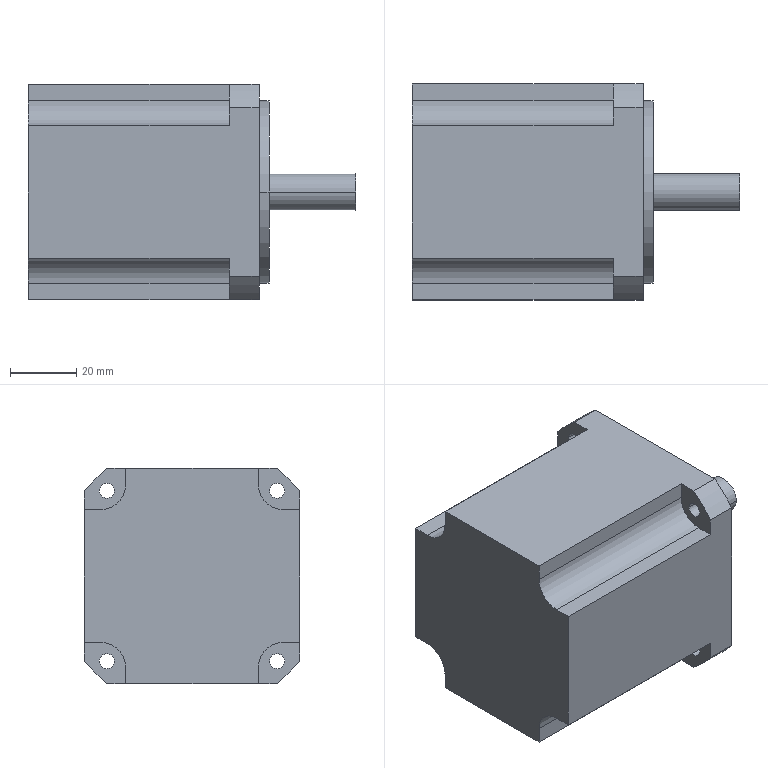Part | STEP file | 2026.6.15-Main Assembly图.sldasm-Part-113 | 1 solid | 40 faces | box 98.5 x 65 x 65 mm | volume 266939 mm3 | cylinder 20 | plane 20 | commonest cylinder face diameters 4.5 x8 15 x4 82.5 x4 11 x2 55 x2
STEP:
#1=CARTESIAN_POINT('',(-1698.224,586.801,4296.167));
#2=VERTEX_POINT('',#1);
#3=CARTESIAN_POINT('',(-1698.224,531.801,4296.167));
#4=VERTEX_POINT('',#3);
#5=CARTESIAN_POINT('',(-1698.224,559.301,4296.167));
#6=DIRECTION('',(1.,0.,0.));
#7=DIRECTION('',(0.,-1.,0.));
#8=AXIS2_PLACEMENT_3D('',#5,#6,#7);
#9=CIRCLE('',#8,27.5);
#10=EDGE_CURVE('',#2,#4,#9,.T.);
#11=ORIENTED_EDGE('',*,*,#10,.T.);
#12=CARTESIAN_POINT('',(-1695.224,531.801,4296.167));
#13=VERTEX_POINT('',#12);
#14=CARTESIAN_POINT('',(-1698.224,531.801,4296.167));
#15=DIRECTION('',(1.,0.,0.));
#16=VECTOR('',#15,1000.);
#17=LINE('',#14,#16);
#18=EDGE_CURVE('',#4,#13,#17,.T.);
#19=ORIENTED_EDGE('',*,*,#18,.T.);
#20=CARTESIAN_POINT('',(-1695.224,586.801,4296.167));
#21=VERTEX_POINT('',#20);
#22=CARTESIAN_POINT('',(-1695.224,559.301,4296.167));
#23=DIRECTION('',(1.,0.,0.));
#24=DIRECTION('',(0.,-1.,0.));
#25=AXIS2_PLACEMENT_3D('',#22,#23,#24);
#26=CIRCLE('',#25,27.5);
#27=EDGE_CURVE('',#21,#13,#26,.T.);
#28=ORIENTED_EDGE('',*,*,#27,.F.);
#29=CARTESIAN_POINT('',(-1698.224,586.801,4296.167));
#30=DIRECTION('',(1.,0.,0.));
#31=VECTOR('',#30,1000.);
#32=LINE('',#29,#31);
#33=EDGE_CURVE('',#2,#21,#32,.T.);
#34=ORIENTED_EDGE('',*,*,#33,.F.);
#35=EDGE_LOOP('',(#11,#19,#28,#34));
#36=FACE_OUTER_BOUND('',#35,.T.);
#37=CARTESIAN_POINT('',(-1698.224,559.301,4296.167));
#38=DIRECTION('',(1.,0.,0.));
#39=DIRECTION('',(0.,1.,0.));
#40=AXIS2_PLACEMENT_3D('',#37,#38,#39);
#41=CYLINDRICAL_SURFACE('',#40,27.5);
#42=ADVANCED_FACE('',(#36),#41,.T.);
#43=CARTESIAN_POINT('',(-1707.224,531.419,4270.534));
#44=VERTEX_POINT('',#43);
#45=CARTESIAN_POINT('',(-1707.224,535.919,4270.534));
#46=VERTEX_POINT('',#45);
#47=CARTESIAN_POINT('',(-1707.224,533.669,4270.534));
#48=DIRECTION('',(1.,0.,0.));
#49=DIRECTION('',(0.,1.,0.));
#50=AXIS2_PLACEMENT_3D('',#47,#48,#49);
#51=CIRCLE('',#50,2.25);
#52=EDGE_CURVE('',#44,#46,#51,.T.);
#53=ORIENTED_EDGE('',*,*,#52,.F.);
#54=CARTESIAN_POINT('',(-1698.224,531.419,4270.534));
#55=VERTEX_POINT('',#54);
#56=CARTESIAN_POINT('',(-1707.224,531.419,4270.534));
#57=DIRECTION('',(1.,0.,0.));
#58=VECTOR('',#57,1000.);
#59=LINE('',#56,#58);
#60=EDGE_CURVE('',#44,#55,#59,.T.);
#61=ORIENTED_EDGE('',*,*,#60,.T.);
#62=CARTESIAN_POINT('',(-1698.224,535.919,4270.534));
#63=VERTEX_POINT('',#62);
#64=CARTESIAN_POINT('',(-1698.224,533.669,4270.534));
#65=DIRECTION('',(1.,0.,0.));
#66=DIRECTION('',(0.,1.,0.));
#67=AXIS2_PLACEMENT_3D('',#64,#65,#66);
#68=CIRCLE('',#67,2.25);
#69=EDGE_CURVE('',#55,#63,#68,.T.);
#70=ORIENTED_EDGE('',*,*,#69,.T.);
#71=CARTESIAN_POINT('',(-1707.224,535.919,4270.534));
#72=DIRECTION('',(1.,0.,0.));
#73=VECTOR('',#72,1000.);
#74=LINE('',#71,#73);
#75=EDGE_CURVE('',#46,#63,#74,.T.);
#76=ORIENTED_EDGE('',*,*,#75,.F.);
#77=EDGE_LOOP('',(#53,#61,#70,#76));
#78=FACE_OUTER_BOUND('',#77,.T.);
#79=CARTESIAN_POINT('',(-1707.224,533.669,4270.534));
#80=DIRECTION('',(1.,0.,0.));
#81=DIRECTION('',(0.,1.,0.));
#82=AXIS2_PLACEMENT_3D('',#79,#80,#81);
#83=CYLINDRICAL_SURFACE('',#82,2.25);
#84=ADVANCED_FACE('',(#78),#83,.F.);
#85=CARTESIAN_POINT('',(-1707.224,582.684,4321.799));
#86=VERTEX_POINT('',#85);
#87=CARTESIAN_POINT('',(-1707.224,587.184,4321.799));
#88=VERTEX_POINT('',#87);
#89=CARTESIAN_POINT('',(-1707.224,584.934,4321.799));
#90=DIRECTION('',(1.,0.,0.));
#91=DIRECTION('',(0.,1.,0.));
#92=AXIS2_PLACEMENT_3D('',#89,#90,#91);
#93=CIRCLE('',#92,2.25);
#94=EDGE_CURVE('',#86,#88,#93,.T.);
#95=ORIENTED_EDGE('',*,*,#94,.F.);
#96=CARTESIAN_POINT('',(-1698.224,582.684,4321.799));
#97=VERTEX_POINT('',#96);
#98=CARTESIAN_POINT('',(-1707.224,582.684,4321.799));
#99=DIRECTION('',(1.,0.,0.));
#100=VECTOR('',#99,1000.);
#101=LINE('',#98,#100);
#102=EDGE_CURVE('',#86,#97,#101,.T.);
#103=ORIENTED_EDGE('',*,*,#102,.T.);
#104=CARTESIAN_POINT('',(-1698.224,587.184,4321.799));
#105=VERTEX_POINT('',#104);
#106=CARTESIAN_POINT('',(-1698.224,584.934,4321.799));
#107=DIRECTION('',(1.,0.,0.));
#108=DIRECTION('',(0.,1.,0.));
#109=AXIS2_PLACEMENT_3D('',#106,#107,#108);
#110=CIRCLE('',#109,2.25);
#111=EDGE_CURVE('',#97,#105,#110,.T.);
#112=ORIENTED_EDGE('',*,*,#111,.T.);
#113=CARTESIAN_POINT('',(-1707.224,587.184,4321.799));
#114=DIRECTION('',(1.,0.,0.));
#115=VECTOR('',#114,1000.);
#116=LINE('',#113,#115);
#117=EDGE_CURVE('',#88,#105,#116,.T.);
#118=ORIENTED_EDGE('',*,*,#117,.F.);
#119=EDGE_LOOP('',(#95,#103,#112,#118));
#120=FACE_OUTER_BOUND('',#119,.T.);
#121=CARTESIAN_POINT('',(-1707.224,584.934,4321.799));
#122=DIRECTION('',(1.,0.,0.));
#123=DIRECTION('',(0.,1.,0.));
#124=AXIS2_PLACEMENT_3D('',#121,#122,#123);
#125=CYLINDRICAL_SURFACE('',#124,2.25);
#126=ADVANCED_FACE('',(#120),#125,.F.);
#127=CARTESIAN_POINT('',(-1707.224,531.419,4321.799));
#128=VERTEX_POINT('',#127);
#129=CARTESIAN_POINT('',(-1707.224,535.919,4321.799));
#130=VERTEX_POINT('',#129);
#131=CARTESIAN_POINT('',(-1707.224,533.669,4321.799));
#132=DIRECTION('',(1.,0.,0.));
#133=DIRECTION('',(0.,1.,0.));
#134=AXIS2_PLACEMENT_3D('',#131,#132,#133);
#135=CIRCLE('',#134,2.25);
#136=EDGE_CURVE('',#128,#130,#135,.T.);
#137=ORIENTED_EDGE('',*,*,#136,.F.);
#138=CARTESIAN_POINT('',(-1698.224,531.419,4321.799));
#139=VERTEX_POINT('',#138);
#140=CARTESIAN_POINT('',(-1707.224,531.419,4321.799));
#141=DIRECTION('',(1.,0.,0.));
#142=VECTOR('',#141,1000.);
#143=LINE('',#140,#142);
#144=EDGE_CURVE('',#128,#139,#143,.T.);
#145=ORIENTED_EDGE('',*,*,#144,.T.);
#146=CARTESIAN_POINT('',(-1698.224,535.919,4321.799));
#147=VERTEX_POINT('',#146);
#148=CARTESIAN_POINT('',(-1698.224,533.669,4321.799));
#149=DIRECTION('',(1.,0.,0.));
#150=DIRECTION('',(0.,1.,0.));
#151=AXIS2_PLACEMENT_3D('',#148,#149,#150);
#152=CIRCLE('',#151,2.25);
#153=EDGE_CURVE('',#139,#147,#152,.T.);
#154=ORIENTED_EDGE('',*,*,#153,.T.);
#155=CARTESIAN_POINT('',(-1707.224,535.919,4321.799));
#156=DIRECTION('',(1.,0.,0.));
#157=VECTOR('',#156,1000.);
#158=LINE('',#155,#157);
#159=EDGE_CURVE('',#130,#147,#158,.T.);
#160=ORIENTED_EDGE('',*,*,#159,.F.);
#161=EDGE_LOOP('',(#137,#145,#154,#160));
#162=FACE_OUTER_BOUND('',#161,.T.);
#163=CARTESIAN_POINT('',(-1707.224,533.669,4321.799));
#164=DIRECTION('',(1.,0.,0.));
#165=DIRECTION('',(0.,1.,0.));
#166=AXIS2_PLACEMENT_3D('',#163,#164,#165);
#167=CYLINDRICAL_SURFACE('',#166,2.25);
#168=ADVANCED_FACE('',(#162),#167,.F.);
#169=CARTESIAN_POINT('',(-1707.224,582.684,4270.534));
#170=VERTEX_POINT('',#169);
#171=CARTESIAN_POINT('',(-1707.224,587.184,4270.534));
#172=VERTEX_POINT('',#171);
#173=CARTESIAN_POINT('',(-1707.224,584.934,4270.534));
#174=DIRECTION('',(1.,0.,0.));
#175=DIRECTION('',(0.,1.,0.));
#176=AXIS2_PLACEMENT_3D('',#173,#174,#175);
#177=CIRCLE('',#176,2.25);
#178=EDGE_CURVE('',#170,#172,#177,.T.);
#179=ORIENTED_EDGE('',*,*,#178,.F.);
#180=CARTESIAN_POINT('',(-1698.224,582.684,4270.534));
#181=VERTEX_POINT('',#180);
#182=CARTESIAN_POINT('',(-1707.224,582.684,4270.534));
#183=DIRECTION('',(1.,0.,0.));
#184=VECTOR('',#183,1000.);
#185=LINE('',#182,#184);
#186=EDGE_CURVE('',#170,#181,#185,.T.);
#187=ORIENTED_EDGE('',*,*,#186,.T.);
#188=CARTESIAN_POINT('',(-1698.224,587.184,4270.534));
#189=VERTEX_POINT('',#188);
#190=CARTESIAN_POINT('',(-1698.224,584.934,4270.534));
#191=DIRECTION('',(1.,0.,0.));
#192=DIRECTION('',(0.,1.,0.));
#193=AXIS2_PLACEMENT_3D('',#190,#191,#192);
#194=CIRCLE('',#193,2.25);
#195=EDGE_CURVE('',#181,#189,#194,.T.);
#196=ORIENTED_EDGE('',*,*,#195,.T.);
#197=CARTESIAN_POINT('',(-1707.224,587.184,4270.534));
#198=DIRECTION('',(1.,0.,0.));
#199=VECTOR('',#198,1000.);
#200=LINE('',#197,#199);
#201=EDGE_CURVE('',#172,#189,#200,.T.);
#202=ORIENTED_EDGE('',*,*,#201,.F.);
#203=EDGE_LOOP('',(#179,#187,#196,#202));
#204=FACE_OUTER_BOUND('',#203,.T.);
#205=CARTESIAN_POINT('',(-1707.224,584.934,4270.534));
#206=DIRECTION('',(1.,0.,0.));
#207=DIRECTION('',(0.,1.,0.));
#208=AXIS2_PLACEMENT_3D('',#205,#206,#207);
#209=CYLINDRICAL_SURFACE('',#208,2.25);
#210=ADVANCED_FACE('',(#204),#209,.F.);
#211=CARTESIAN_POINT('',(-1669.224,553.801,4296.167));
#212=VERTEX_POINT('',#211);
#213=CARTESIAN_POINT('',(-1669.224,564.801,4296.167));
#214=VERTEX_POINT('',#213);
#215=CARTESIAN_POINT('',(-1669.224,559.301,4296.167));
#216=DIRECTION('',(-1.,0.,0.));
#217=DIRECTION('',(0.,0.,1.));
#218=AXIS2_PLACEMENT_3D('',#215,#216,#217);
#219=CIRCLE('',#218,5.5);
#220=EDGE_CURVE('',#212,#214,#219,.T.);
#221=ORIENTED_EDGE('',*,*,#220,.T.);
#222=CARTESIAN_POINT('',(-1695.224,564.801,4296.167));
#223=VERTEX_POINT('',#222);
#224=CARTESIAN_POINT('',(-1669.224,564.801,4296.167));
#225=DIRECTION('',(-1.,0.,0.));
#226=VECTOR('',#225,1000.);
#227=LINE('',#224,#226);
#228=EDGE_CURVE('',#214,#223,#227,.T.);
#229=ORIENTED_EDGE('',*,*,#228,.T.);
#230=CARTESIAN_POINT('',(-1695.224,553.801,4296.167));
#231=VERTEX_POINT('',#230);
#232=CARTESIAN_POINT('',(-1695.224,559.301,4296.167));
#233=DIRECTION('',(-1.,0.,0.));
#234=DIRECTION('',(0.,0.,1.));
#235=AXIS2_PLACEMENT_3D('',#232,#233,#234);
#236=CIRCLE('',#235,5.5);
#237=EDGE_CURVE('',#231,#223,#236,.T.);
#238=ORIENTED_EDGE('',*,*,#237,.F.);
#239=CARTESIAN_POINT('',(-1669.224,553.801,4296.167));
#240=DIRECTION('',(-1.,0.,0.));
#241=VECTOR('',#240,1000.);
#242=LINE('',#239,#241);
#243=EDGE_CURVE('',#212,#231,#242,.T.);
#244=ORIENTED_EDGE('',*,*,#243,.F.);
#245=EDGE_LOOP('',(#221,#229,#238,#244));
#246=FACE_OUTER_BOUND('',#245,.T.);
#247=CARTESIAN_POINT('',(-1669.224,559.301,4296.167));
#248=DIRECTION('',(-1.,0.,0.));
#249=DIRECTION('',(0.,-1.,0.));
#250=AXIS2_PLACEMENT_3D('',#247,#248,#249);
#251=CYLINDRICAL_SURFACE('',#250,5.5);
#252=ADVANCED_FACE('',(#246),#251,.T.);
#253=ORIENTED_EDGE('',*,*,#228,.F.);
#254=CARTESIAN_POINT('',(-1669.224,559.301,4296.167));
#255=DIRECTION('',(-1.,0.,0.));
#256=DIRECTION('',(0.,0.,1.));
#257=AXIS2_PLACEMENT_3D('',#254,#255,#256);
#258=CIRCLE('',#257,5.5);
#259=EDGE_CURVE('',#214,#212,#258,.T.);
#260=ORIENTED_EDGE('',*,*,#259,.T.);
#261=ORIENTED_EDGE('',*,*,#243,.T.);
#262=CARTESIAN_POINT('',(-1695.224,559.301,4296.167));
#263=DIRECTION('',(-1.,0.,0.));
#264=DIRECTION('',(0.,0.,1.));
#265=AXIS2_PLACEMENT_3D('',#262,#263,#264);
#266=CIRCLE('',#265,5.5);
#267=EDGE_CURVE('',#223,#231,#266,.T.);
#268=ORIENTED_EDGE('',*,*,#267,.F.);
#269=EDGE_LOOP('',(#253,#260,#261,#268));
#270=FACE_OUTER_BOUND('',#269,.T.);
#271=CARTESIAN_POINT('',(-1669.224,559.301,4296.167));
#272=DIRECTION('',(-1.,0.,0.));
#273=DIRECTION('',(0.,-1.,0.));
#274=AXIS2_PLACEMENT_3D('',#271,#272,#273);
#275=CYLINDRICAL_SURFACE('',#274,5.5);
#276=ADVANCED_FACE('',(#270),#275,.T.);
#277=ORIENTED_EDGE('',*,*,#220,.F.);
#278=ORIENTED_EDGE('',*,*,#259,.F.);
#279=EDGE_LOOP('',(#277,#278));
#280=FACE_OUTER_BOUND('',#279,.T.);
#281=CARTESIAN_POINT('',(-1669.224,559.301,4296.167));
#282=DIRECTION('',(-1.,0.,0.));
#283=DIRECTION('',(0.,-1.,0.));
#284=AXIS2_PLACEMENT_3D('',#281,#282,#283);
#285=PLANE('',#284);
#286=ADVANCED_FACE('',(#280),#285,.F.);
#287=CARTESIAN_POINT('',(-1707.224,579.301,4268.667));
#288=VERTEX_POINT('',#287);
#289=CARTESIAN_POINT('',(-1707.224,579.301,4263.667));
#290=VERTEX_POINT('',#289);
#291=CARTESIAN_POINT('',(-1707.224,579.301,4268.667));
#292=DIRECTION('',(0.,0.,-1.));
#293=VECTOR('',#292,1000.);
#294=LINE('',#291,#293);
#295=EDGE_CURVE('',#288,#290,#294,.T.);
#296=ORIENTED_EDGE('',*,*,#295,.F.);
#297=CARTESIAN_POINT('',(-1707.224,586.801,4276.167));
#298=VERTEX_POINT('',#297);
#299=CARTESIAN_POINT('',(-1707.224,586.801,4268.667));
#300=DIRECTION('',(1.,0.,0.));
#301=DIRECTION('',(0.,-1.,0.));
#302=AXIS2_PLACEMENT_3D('',#299,#300,#301);
#303=CIRCLE('',#302,7.5);
#304=EDGE_CURVE('',#298,#288,#303,.T.);
#305=ORIENTED_EDGE('',*,*,#304,.F.);
#306=CARTESIAN_POINT('',(-1707.224,591.801,4276.167));
#307=VERTEX_POINT('',#306);
#308=CARTESIAN_POINT('',(-1707.224,591.801,4276.167));
#309=DIRECTION('',(0.,-1.,0.));
#310=VECTOR('',#309,1000.);
#311=LINE('',#308,#310);
#312=EDGE_CURVE('',#307,#298,#311,.T.);
#313=ORIENTED_EDGE('',*,*,#312,.F.);
#314=CARTESIAN_POINT('',(-1707.224,591.801,4270.764));
#315=VERTEX_POINT('',#314);
#316=CARTESIAN_POINT('',(-1707.224,591.801,4321.57));
#317=DIRECTION('',(0.,0.,-1.));
#318=VECTOR('',#317,1000.);
#319=LINE('',#316,#318);
#320=EDGE_CURVE('',#307,#315,#319,.T.);
#321=ORIENTED_EDGE('',*,*,#320,.T.);
#322=CARTESIAN_POINT('',(-1707.224,584.704,4263.667));
#323=VERTEX_POINT('',#322);
#324=CARTESIAN_POINT('',(-1707.224,559.301,4296.167));
#325=DIRECTION('',(-1.,0.,0.));
#326=DIRECTION('',(0.,0.,1.));
#327=AXIS2_PLACEMENT_3D('',#324,#325,#326);
#328=CIRCLE('',#327,41.25);
#329=EDGE_CURVE('',#315,#323,#328,.T.);
#330=ORIENTED_EDGE('',*,*,#329,.T.);
#331=CARTESIAN_POINT('',(-1707.224,584.704,4263.667));
#332=DIRECTION('',(0.,-1.,0.));
#333=VECTOR('',#332,1000.);
#334=LINE('',#331,#333);
#335=EDGE_CURVE('',#323,#290,#334,.T.);
#336=ORIENTED_EDGE('',*,*,#335,.T.);
#337=EDGE_LOOP('',(#296,#305,#313,#321,#330,#336));
#338=FACE_OUTER_BOUND('',#337,.T.);
#339=CARTESIAN_POINT('',(-1707.224,584.934,4270.534));
#340=DIRECTION('',(1.,0.,0.));
#341=DIRECTION('',(0.,1.,0.));
#342=AXIS2_PLACEMENT_3D('',#339,#340,#341);
#343=CIRCLE('',#342,2.25);
#344=EDGE_CURVE('',#172,#170,#343,.T.);
#345=ORIENTED_EDGE('',*,*,#344,.T.);
#346=ORIENTED_EDGE('',*,*,#178,.T.);
#347=EDGE_LOOP('',(#345,#346));
#348=FACE_BOUND('',#347,.T.);
#349=CARTESIAN_POINT('',(-1707.224,559.301,4296.167));
#350=DIRECTION('',(-1.,0.,0.));
#351=DIRECTION('',(0.,-1.,0.));
#352=AXIS2_PLACEMENT_3D('',#349,#350,#351);
#353=PLANE('',#352);
#354=ADVANCED_FACE('',(#338,#348),#353,.T.);
#355=CARTESIAN_POINT('',(-1707.224,586.801,4316.167));
#356=VERTEX_POINT('',#355);
#357=CARTESIAN_POINT('',(-1707.224,591.801,4316.167));
#358=VERTEX_POINT('',#357);
#359=CARTESIAN_POINT('',(-1707.224,586.801,4316.167));
#360=DIRECTION('',(0.,1.,0.));
#361=VECTOR('',#360,1000.);
#362=LINE('',#359,#361);
#363=EDGE_CURVE('',#356,#358,#362,.T.);
#364=ORIENTED_EDGE('',*,*,#363,.F.);
#365=CARTESIAN_POINT('',(-1707.224,579.301,4323.667));
#366=VERTEX_POINT('',#365);
#367=CARTESIAN_POINT('',(-1707.224,586.801,4323.667));
#368=DIRECTION('',(1.,0.,0.));
#369=DIRECTION('',(0.,1.,0.));
#370=AXIS2_PLACEMENT_3D('',#367,#368,#369);
#371=CIRCLE('',#370,7.5);
#372=EDGE_CURVE('',#366,#356,#371,.T.);
#373=ORIENTED_EDGE('',*,*,#372,.F.);
#374=CARTESIAN_POINT('',(-1707.224,579.301,4328.667));
#375=VERTEX_POINT('',#374);
#376=CARTESIAN_POINT('',(-1707.224,579.301,4328.667));
#377=DIRECTION('',(0.,0.,-1.));
#378=VECTOR('',#377,1000.);
#379=LINE('',#376,#378);
#380=EDGE_CURVE('',#375,#366,#379,.T.);
#381=ORIENTED_EDGE('',*,*,#380,.F.);
#382=CARTESIAN_POINT('',(-1707.224,584.704,4328.667));
#383=VERTEX_POINT('',#382);
#384=CARTESIAN_POINT('',(-1707.224,533.898,4328.667));
#385=DIRECTION('',(0.,1.,0.));
#386=VECTOR('',#385,1000.);
#387=LINE('',#384,#386);
#388=EDGE_CURVE('',#375,#383,#387,.T.);
#389=ORIENTED_EDGE('',*,*,#388,.T.);
#390=CARTESIAN_POINT('',(-1707.224,591.801,4321.57));
#391=VERTEX_POINT('',#390);
#392=CARTESIAN_POINT('',(-1707.224,559.301,4296.167));
#393=DIRECTION('',(-1.,0.,0.));
#394=DIRECTION('',(0.,0.,1.));
#395=AXIS2_PLACEMENT_3D('',#392,#393,#394);
#396=CIRCLE('',#395,41.25);
#397=EDGE_CURVE('',#383,#391,#396,.T.);
#398=ORIENTED_EDGE('',*,*,#397,.T.);
#399=CARTESIAN_POINT('',(-1707.224,591.801,4321.57));
#400=DIRECTION('',(0.,0.,-1.));
#401=VECTOR('',#400,1000.);
#402=LINE('',#399,#401);
#403=EDGE_CURVE('',#391,#358,#402,.T.);
#404=ORIENTED_EDGE('',*,*,#403,.T.);
#405=EDGE_LOOP('',(#364,#373,#381,#389,#398,#404));
#406=FACE_OUTER_BOUND('',#405,.T.);
#407=CARTESIAN_POINT('',(-1707.224,584.934,4321.799));
#408=DIRECTION('',(1.,0.,0.));
#409=DIRECTION('',(0.,1.,0.));
#410=AXIS2_PLACEMENT_3D('',#407,#408,#409);
#411=CIRCLE('',#410,2.25);
#412=EDGE_CURVE('',#88,#86,#411,.T.);
#413=ORIENTED_EDGE('',*,*,#412,.T.);
#414=ORIENTED_EDGE('',*,*,#94,.T.);
#415=EDGE_LOOP('',(#413,#414));
#416=FACE_BOUND('',#415,.T.);
#417=CARTESIAN_POINT('',(-1707.224,559.301,4296.167));
#418=DIRECTION('',(-1.,0.,0.));
#419=DIRECTION('',(0.,-1.,0.));
#420=AXIS2_PLACEMENT_3D('',#417,#418,#419);
#421=PLANE('',#420);
#422=ADVANCED_FACE('',(#406,#416),#421,.T.);
#423=CARTESIAN_POINT('',(-1707.224,539.301,4323.667));
#424=VERTEX_POINT('',#423);
#425=CARTESIAN_POINT('',(-1707.224,539.301,4328.667));
#426=VERTEX_POINT('',#425);
#427=CARTESIAN_POINT('',(-1707.224,539.301,4323.667));
#428=DIRECTION('',(0.,0.,1.));
#429=VECTOR('',#428,1000.);
#430=LINE('',#427,#429);
#431=EDGE_CURVE('',#424,#426,#430,.T.);
#432=ORIENTED_EDGE('',*,*,#431,.F.);
#433=CARTESIAN_POINT('',(-1707.224,531.801,4316.167));
#434=VERTEX_POINT('',#433);
#435=CARTESIAN_POINT('',(-1707.224,531.801,4323.667));
#436=DIRECTION('',(1.,0.,0.));
#437=DIRECTION('',(0.,-1.,0.));
#438=AXIS2_PLACEMENT_3D('',#435,#436,#437);
#439=CIRCLE('',#438,7.5);
#440=EDGE_CURVE('',#434,#424,#439,.T.);
#441=ORIENTED_EDGE('',*,*,#440,.F.);
#442=CARTESIAN_POINT('',(-1707.224,526.801,4316.167));
#443=VERTEX_POINT('',#442);
#444=CARTESIAN_POINT('',(-1707.224,526.801,4316.167));
#445=DIRECTION('',(0.,1.,0.));
#446=VECTOR('',#445,1000.);
#447=LINE('',#444,#446);
#448=EDGE_CURVE('',#443,#434,#447,.T.);
#449=ORIENTED_EDGE('',*,*,#448,.F.);
#450=CARTESIAN_POINT('',(-1707.224,526.801,4321.57));
#451=VERTEX_POINT('',#450);
#452=CARTESIAN_POINT('',(-1707.224,526.801,4270.764));
#453=DIRECTION('',(0.,0.,1.));
#454=VECTOR('',#453,1000.);
#455=LINE('',#452,#454);
#456=EDGE_CURVE('',#443,#451,#455,.T.);
#457=ORIENTED_EDGE('',*,*,#456,.T.);
#458=CARTESIAN_POINT('',(-1707.224,533.898,4328.667));
#459=VERTEX_POINT('',#458);
#460=CARTESIAN_POINT('',(-1707.224,559.301,4296.167));
#461=DIRECTION('',(-1.,0.,0.));
#462=DIRECTION('',(0.,0.,1.));
#463=AXIS2_PLACEMENT_3D('',#460,#461,#462);
#464=CIRCLE('',#463,41.25);
#465=EDGE_CURVE('',#451,#459,#464,.T.);
#466=ORIENTED_EDGE('',*,*,#465,.T.);
#467=CARTESIAN_POINT('',(-1707.224,533.898,4328.667));
#468=DIRECTION('',(0.,1.,0.));
#469=VECTOR('',#468,1000.);
#470=LINE('',#467,#469);
#471=EDGE_CURVE('',#459,#426,#470,.T.);
#472=ORIENTED_EDGE('',*,*,#471,.T.);
#473=EDGE_LOOP('',(#432,#441,#449,#457,#466,#472));
#474=FACE_OUTER_BOUND('',#473,.T.);
#475=CARTESIAN_POINT('',(-1707.224,533.669,4321.799));
#476=DIRECTION('',(1.,0.,0.));
#477=DIRECTION('',(0.,1.,0.));
#478=AXIS2_PLACEMENT_3D('',#475,#476,#477);
#479=CIRCLE('',#478,2.25);
#480=EDGE_CURVE('',#130,#128,#479,.T.);
#481=ORIENTED_EDGE('',*,*,#480,.T.);
#482=ORIENTED_EDGE('',*,*,#136,.T.);
#483=EDGE_LOOP('',(#481,#482));
#484=FACE_BOUND('',#483,.T.);
#485=CARTESIAN_POINT('',(-1707.224,559.301,4296.167));
#486=DIRECTION('',(-1.,0.,0.));
#487=DIRECTION('',(0.,-1.,0.));
#488=AXIS2_PLACEMENT_3D('',#485,#486,#487);
#489=PLANE('',#488);
#490=ADVANCED_FACE('',(#474,#484),#489,.T.);
#491=CARTESIAN_POINT('',(-1698.224,526.801,4270.764));
#492=VERTEX_POINT('',#491);
#493=CARTESIAN_POINT('',(-1698.224,526.801,4321.57));
#494=VERTEX_POINT('',#493);
#495=CARTESIAN_POINT('',(-1698.224,526.801,4270.764));
#496=DIRECTION('',(0.,0.,1.));
#497=VECTOR('',#496,1000.);
#498=LINE('',#495,#497);
#499=EDGE_CURVE('',#492,#494,#498,.T.);
#500=ORIENTED_EDGE('',*,*,#499,.T.);
#501=CARTESIAN_POINT('',(-1707.224,526.801,4321.57));
#502=DIRECTION('',(1.,0.,0.));
#503=VECTOR('',#502,1000.);
#504=LINE('',#501,#503);
#505=EDGE_CURVE('',#451,#494,#504,.T.);
#506=ORIENTED_EDGE('',*,*,#505,.F.);
#507=ORIENTED_EDGE('',*,*,#456,.F.);
#508=CARTESIAN_POINT('',(-1767.724,526.801,4316.167));
#509=VERTEX_POINT('',#508);
#510=CARTESIAN_POINT('',(-1767.724,526.801,4316.167));
#511=DIRECTION('',(1.,0.,0.));
#512=VECTOR('',#511,1000.);
#513=LINE('',#510,#512);
#514=EDGE_CURVE('',#509,#443,#513,.T.);
#515=ORIENTED_EDGE('',*,*,#514,.F.);
#516=CARTESIAN_POINT('',(-1767.724,526.801,4276.167));
#517=VERTEX_POINT('',#516);
#518=CARTESIAN_POINT('',(-1767.724,526.801,4276.167));
#519=DIRECTION('',(0.,0.,1.));
#520=VECTOR('',#519,1000.);
#521=LINE('',#518,#520);
#522=EDGE_CURVE('',#517,#509,#521,.T.);
#523=ORIENTED_EDGE('',*,*,#522,.F.);
#524=CARTESIAN_POINT('',(-1707.224,526.801,4276.167));
#525=VERTEX_POINT('',#524);
#526=CARTESIAN_POINT('',(-1767.724,526.801,4276.167));
#527=DIRECTION('',(1.,0.,0.));
#528=VECTOR('',#527,1000.);
#529=LINE('',#526,#528);
#530=EDGE_CURVE('',#517,#525,#529,.T.);
#531=ORIENTED_EDGE('',*,*,#530,.T.);
#532=CARTESIAN_POINT('',(-1707.224,526.801,4270.764));
#533=VERTEX_POINT('',#532);
#534=CARTESIAN_POINT('',(-1707.224,526.801,4270.764));
#535=DIRECTION('',(0.,0.,1.));
#536=VECTOR('',#535,1000.);
#537=LINE('',#534,#536);
#538=EDGE_CURVE('',#533,#525,#537,.T.);
#539=ORIENTED_EDGE('',*,*,#538,.F.);
#540=CARTESIAN_POINT('',(-1707.224,526.801,4270.764));
#541=DIRECTION('',(1.,0.,0.));
#542=VECTOR('',#541,1000.);
#543=LINE('',#540,#542);
#544=EDGE_CURVE('',#533,#492,#543,.T.);
#545=ORIENTED_EDGE('',*,*,#544,.T.);
#546=EDGE_LOOP('',(#500,#506,#507,#515,#523,#531,#539,#545));
#547=FACE_OUTER_BOUND('',#546,.T.);
#548=CARTESIAN_POINT('',(-1707.224,526.801,4270.764));
#549=DIRECTION('',(0.,1.,0.));
#550=DIRECTION('',(0.,0.,1.));
#551=AXIS2_PLACEMENT_3D('',#548,#549,#550);
#552=PLANE('',#551);
#553=ADVANCED_FACE('',(#547),#552,.F.);
#554=CARTESIAN_POINT('',(-1698.224,533.898,4328.667));
#555=VERTEX_POINT('',#554);
#556=CARTESIAN_POINT('',(-1698.224,559.301,4296.167));
#557=DIRECTION('',(-1.,0.,0.));
#558=DIRECTION('',(0.,0.,1.));
#559=AXIS2_PLACEMENT_3D('',#556,#557,#558);
#560=CIRCLE('',#559,41.25);
#561=EDGE_CURVE('',#494,#555,#560,.T.);
#562=ORIENTED_EDGE('',*,*,#561,.T.);
#563=CARTESIAN_POINT('',(-1707.224,533.898,4328.667));
#564=DIRECTION('',(1.,0.,0.));
#565=VECTOR('',#564,1000.);
#566=LINE('',#563,#565);
#567=EDGE_CURVE('',#459,#555,#566,.T.);
#568=ORIENTED_EDGE('',*,*,#567,.F.);
#569=ORIENTED_EDGE('',*,*,#465,.F.);
#570=ORIENTED_EDGE('',*,*,#505,.T.);
#571=EDGE_LOOP('',(#562,#568,#569,#570));
#572=FACE_OUTER_BOUND('',#571,.T.);
#573=CARTESIAN_POINT('',(-1707.224,559.301,4296.167));
#574=DIRECTION('',(1.,0.,0.));
#575=DIRECTION('',(0.,1.,0.));
#576=AXIS2_PLACEMENT_3D('',#573,#574,#575);
#577=CYLINDRICAL_SURFACE('',#576,41.25);
#578=ADVANCED_FACE('',(#572),#577,.T.);
#579=CARTESIAN_POINT('',(-1698.224,584.704,4328.667));
#580=VERTEX_POINT('',#579);
#581=CARTESIAN_POINT('',(-1698.224,533.898,4328.667));
#582=DIRECTION('',(0.,1.,0.));
#583=VECTOR('',#582,1000.);
#584=LINE('',#581,#583);
#585=EDGE_CURVE('',#555,#580,#584,.T.);
#586=ORIENTED_EDGE('',*,*,#585,.T.);
#587=CARTESIAN_POINT('',(-1707.224,584.704,4328.667));
#588=DIRECTION('',(1.,0.,0.));
#589=VECTOR('',#588,1000.);
#590=LINE('',#587,#589);
#591=EDGE_CURVE('',#383,#580,#590,.T.);
#592=ORIENTED_EDGE('',*,*,#591,.F.);
#593=ORIENTED_EDGE('',*,*,#388,.F.);
#594=CARTESIAN_POINT('',(-1767.724,579.301,4328.667));
#595=VERTEX_POINT('',#594);
#596=CARTESIAN_POINT('',(-1767.724,579.301,4328.667));
#597=DIRECTION('',(1.,0.,0.));
#598=VECTOR('',#597,1000.);
#599=LINE('',#596,#598);
#600=EDGE_CURVE('',#595,#375,#599,.T.);
#601=ORIENTED_EDGE('',*,*,#600,.F.);
#602=CARTESIAN_POINT('',(-1767.724,539.301,4328.667));
#603=VERTEX_POINT('',#602);
#604=CARTESIAN_POINT('',(-1767.724,539.301,4328.667));
#605=DIRECTION('',(0.,1.,0.));
#606=VECTOR('',#605,1000.);
#607=LINE('',#604,#606);
#608=EDGE_CURVE('',#603,#595,#607,.T.);
#609=ORIENTED_EDGE('',*,*,#608,.F.);
#610=CARTESIAN_POINT('',(-1767.724,539.301,4328.667));
#611=DIRECTION('',(1.,0.,0.));
#612=VECTOR('',#611,1000.);
#613=LINE('',#610,#612);
#614=EDGE_CURVE('',#603,#426,#613,.T.);
#615=ORIENTED_EDGE('',*,*,#614,.T.);
#616=ORIENTED_EDGE('',*,*,#471,.F.);
#617=ORIENTED_EDGE('',*,*,#567,.T.);
#618=EDGE_LOOP('',(#586,#592,#593,#601,#609,#615,#616,#617));
#619=FACE_OUTER_BOUND('',#618,.T.);
#620=CARTESIAN_POINT('',(-1707.224,533.898,4328.667));
#621=DIRECTION('',(0.,0.,-1.));
#622=DIRECTION('',(0.,1.,0.));
#623=AXIS2_PLACEMENT_3D('',#620,#621,#622);
#624=PLANE('',#623);
#625=ADVANCED_FACE('',(#619),#624,.F.);
#626=CARTESIAN_POINT('',(-1698.224,591.801,4321.57));
#627=VERTEX_POINT('',#626);
#628=CARTESIAN_POINT('',(-1698.224,559.301,4296.167));
#629=DIRECTION('',(-1.,0.,0.));
#630=DIRECTION('',(0.,0.,1.));
#631=AXIS2_PLACEMENT_3D('',#628,#629,#630);
#632=CIRCLE('',#631,41.25);
#633=EDGE_CURVE('',#580,#627,#632,.T.);
#634=ORIENTED_EDGE('',*,*,#633,.T.);
#635=CARTESIAN_POINT('',(-1707.224,591.801,4321.57));
#636=DIRECTION('',(1.,0.,0.));
#637=VECTOR('',#636,1000.);
#638=LINE('',#635,#637);
#639=EDGE_CURVE('',#391,#627,#638,.T.);
#640=ORIENTED_EDGE('',*,*,#639,.F.);
#641=ORIENTED_EDGE('',*,*,#397,.F.);
#642=ORIENTED_EDGE('',*,*,#591,.T.);
#643=EDGE_LOOP('',(#634,#640,#641,#642));
#644=FACE_OUTER_BOUND('',#643,.T.);
#645=CARTESIAN_POINT('',(-1707.224,559.301,4296.167));
#646=DIRECTION('',(1.,0.,0.));
#647=DIRECTION('',(0.,1.,0.));
#648=AXIS2_PLACEMENT_3D('',#645,#646,#647);
#649=CYLINDRICAL_SURFACE('',#648,41.25);
#650=ADVANCED_FACE('',(#644),#649,.T.);
#651=CARTESIAN_POINT('',(-1698.224,591.801,4270.764));
#652=VERTEX_POINT('',#651);
#653=CARTESIAN_POINT('',(-1698.224,591.801,4321.57));
#654=DIRECTION('',(0.,0.,-1.));
#655=VECTOR('',#654,1000.);
#656=LINE('',#653,#655);
#657=EDGE_CURVE('',#627,#652,#656,.T.);
#658=ORIENTED_EDGE('',*,*,#657,.T.);
#659=CARTESIAN_POINT('',(-1707.224,591.801,4270.764));
#660=DIRECTION('',(1.,0.,0.));
#661=VECTOR('',#660,1000.);
#662=LINE('',#659,#661);
#663=EDGE_CURVE('',#315,#652,#662,.T.);
#664=ORIENTED_EDGE('',*,*,#663,.F.);
#665=ORIENTED_EDGE('',*,*,#320,.F.);
#666=CARTESIAN_POINT('',(-1767.724,591.801,4276.167));
#667=VERTEX_POINT('',#666);
#668=CARTESIAN_POINT('',(-1767.724,591.801,4276.167));
#669=DIRECTION('',(1.,0.,0.));
#670=VECTOR('',#669,1000.);
#671=LINE('',#668,#670);
#672=EDGE_CURVE('',#667,#307,#671,.T.);
#673=ORIENTED_EDGE('',*,*,#672,.F.);
#674=CARTESIAN_POINT('',(-1767.724,591.801,4316.167));
#675=VERTEX_POINT('',#674);
#676=CARTESIAN_POINT('',(-1767.724,591.801,4316.167));
#677=DIRECTION('',(0.,0.,-1.));
#678=VECTOR('',#677,1000.);
#679=LINE('',#676,#678);
#680=EDGE_CURVE('',#675,#667,#679,.T.);
#681=ORIENTED_EDGE('',*,*,#680,.F.);
#682=CARTESIAN_POINT('',(-1767.724,591.801,4316.167));
#683=DIRECTION('',(1.,0.,0.));
#684=VECTOR('',#683,1000.);
#685=LINE('',#682,#684);
#686=EDGE_CURVE('',#675,#358,#685,.T.);
#687=ORIENTED_EDGE('',*,*,#686,.T.);
#688=ORIENTED_EDGE('',*,*,#403,.F.);
#689=ORIENTED_EDGE('',*,*,#639,.T.);
#690=EDGE_LOOP('',(#658,#664,#665,#673,#681,#687,#688,#689));
#691=FACE_OUTER_BOUND('',#690,.T.);
#692=CARTESIAN_POINT('',(-1707.224,591.801,4321.57));
#693=DIRECTION('',(0.,-1.,0.));
#694=DIRECTION('',(0.,0.,-1.));
#695=AXIS2_PLACEMENT_3D('',#692,#693,#694);
#696=PLANE('',#695);
#697=ADVANCED_FACE('',(#691),#696,.F.);
#698=CARTESIAN_POINT('',(-1698.224,584.704,4263.667));
#699=VERTEX_POINT('',#698);
#700=CARTESIAN_POINT('',(-1698.224,559.301,4296.167));
#701=DIRECTION('',(-1.,0.,0.));
#702=DIRECTION('',(0.,0.,1.));
#703=AXIS2_PLACEMENT_3D('',#700,#701,#702);
#704=CIRCLE('',#703,41.25);
#705=EDGE_CURVE('',#652,#699,#704,.T.);
#706=ORIENTED_EDGE('',*,*,#705,.T.);
#707=CARTESIAN_POINT('',(-1707.224,584.704,4263.667));
#708=DIRECTION('',(1.,0.,0.));
#709=VECTOR('',#708,1000.);
#710=LINE('',#707,#709);
#711=EDGE_CURVE('',#323,#699,#710,.T.);
#712=ORIENTED_EDGE('',*,*,#711,.F.);
#713=ORIENTED_EDGE('',*,*,#329,.F.);
#714=ORIENTED_EDGE('',*,*,#663,.T.);
#715=EDGE_LOOP('',(#706,#712,#713,#714));
#716=FACE_OUTER_BOUND('',#715,.T.);
#717=CARTESIAN_POINT('',(-1707.224,559.301,4296.167));
#718=DIRECTION('',(1.,0.,0.));
#719=DIRECTION('',(0.,1.,0.));
#720=AXIS2_PLACEMENT_3D('',#717,#718,#719);
#721=CYLINDRICAL_SURFACE('',#720,41.25);
#722=ADVANCED_FACE('',(#716),#721,.T.);
#723=CARTESIAN_POINT('',(-1698.224,533.898,4263.667));
#724=VERTEX_POINT('',#723);
#725=CARTESIAN_POINT('',(-1698.224,584.704,4263.667));
#726=DIRECTION('',(0.,-1.,0.));
#727=VECTOR('',#726,1000.);
#728=LINE('',#725,#727);
#729=EDGE_CURVE('',#699,#724,#728,.T.);
#730=ORIENTED_EDGE('',*,*,#729,.T.);
#731=CARTESIAN_POINT('',(-1707.224,533.898,4263.667));
#732=VERTEX_POINT('',#731);
#733=CARTESIAN_POINT('',(-1707.224,533.898,4263.667));
#734=DIRECTION('',(1.,0.,0.));
#735=VECTOR('',#734,1000.);
#736=LINE('',#733,#735);
#737=EDGE_CURVE('',#732,#724,#736,.T.);
#738=ORIENTED_EDGE('',*,*,#737,.F.);
#739=CARTESIAN_POINT('',(-1707.224,539.301,4263.667));
#740=VERTEX_POINT('',#739);
#741=CARTESIAN_POINT('',(-1707.224,584.704,4263.667));
#742=DIRECTION('',(0.,-1.,0.));
#743=VECTOR('',#742,1000.);
#744=LINE('',#741,#743);
#745=EDGE_CURVE('',#740,#732,#744,.T.);
#746=ORIENTED_EDGE('',*,*,#745,.F.);
#747=CARTESIAN_POINT('',(-1767.724,539.301,4263.667));
#748=VERTEX_POINT('',#747);
#749=CARTESIAN_POINT('',(-1767.724,539.301,4263.667));
#750=DIRECTION('',(1.,0.,0.));
#751=VECTOR('',#750,1000.);
#752=LINE('',#749,#751);
#753=EDGE_CURVE('',#748,#740,#752,.T.);
#754=ORIENTED_EDGE('',*,*,#753,.F.);
#755=CARTESIAN_POINT('',(-1767.724,579.301,4263.667));
#756=VERTEX_POINT('',#755);
#757=CARTESIAN_POINT('',(-1767.724,579.301,4263.667));
#758=DIRECTION('',(0.,-1.,0.));
#759=VECTOR('',#758,1000.);
#760=LINE('',#757,#759);
#761=EDGE_CURVE('',#756,#748,#760,.T.);
#762=ORIENTED_EDGE('',*,*,#761,.F.);
#763=CARTESIAN_POINT('',(-1767.724,579.301,4263.667));
#764=DIRECTION('',(1.,0.,0.));
#765=VECTOR('',#764,1000.);
#766=LINE('',#763,#765);
#767=EDGE_CURVE('',#756,#290,#766,.T.);
#768=ORIENTED_EDGE('',*,*,#767,.T.);
#769=ORIENTED_EDGE('',*,*,#335,.F.);
#770=ORIENTED_EDGE('',*,*,#711,.T.);
#771=EDGE_LOOP('',(#730,#738,#746,#754,#762,#768,#769,#770));
#772=FACE_OUTER_BOUND('',#771,.T.);
#773=CARTESIAN_POINT('',(-1707.224,584.704,4263.667));
#774=DIRECTION('',(0.,0.,1.));
#775=DIRECTION('',(0.,-1.,0.));
#776=AXIS2_PLACEMENT_3D('',#773,#774,#775);
#777=PLANE('',#776);
#778=ADVANCED_FACE('',(#772),#777,.F.);
#779=ORIENTED_EDGE('',*,*,#186,.F.);
#780=ORIENTED_EDGE('',*,*,#344,.F.);
#781=ORIENTED_EDGE('',*,*,#201,.T.);
#782=CARTESIAN_POINT('',(-1698.224,584.934,4270.534));
#783=DIRECTION('',(1.,0.,0.));
#784=DIRECTION('',(0.,1.,0.));
#785=AXIS2_PLACEMENT_3D('',#782,#783,#784);
#786=CIRCLE('',#785,2.25);
#787=EDGE_CURVE('',#189,#181,#786,.T.);
#788=ORIENTED_EDGE('',*,*,#787,.T.);
#789=EDGE_LOOP('',(#779,#780,#781,#788));
#790=FACE_OUTER_BOUND('',#789,.T.);
#791=CARTESIAN_POINT('',(-1707.224,584.934,4270.534));
#792=DIRECTION('',(1.,0.,0.));
#793=DIRECTION('',(0.,1.,0.));
#794=AXIS2_PLACEMENT_3D('',#791,#792,#793);
#795=CYLINDRICAL_SURFACE('',#794,2.25);
#796=ADVANCED_FACE('',(#790),#795,.F.);
#797=ORIENTED_EDGE('',*,*,#144,.F.);
#798=ORIENTED_EDGE('',*,*,#480,.F.);
#799=ORIENTED_EDGE('',*,*,#159,.T.);
#800=CARTESIAN_POINT('',(-1698.224,533.669,4321.799));
#801=DIRECTION('',(1.,0.,0.));
#802=DIRECTION('',(0.,1.,0.));
#803=AXIS2_PLACEMENT_3D('',#800,#801,#802);
#804=CIRCLE('',#803,2.25);
#805=EDGE_CURVE('',#147,#139,#804,.T.);
#806=ORIENTED_EDGE('',*,*,#805,.T.);
#807=EDGE_LOOP('',(#797,#798,#799,#806));
#808=FACE_OUTER_BOUND('',#807,.T.);
#809=CARTESIAN_POINT('',(-1707.224,533.669,4321.799));
#810=DIRECTION('',(1.,0.,0.));
#811=DIRECTION('',(0.,1.,0.));
#812=AXIS2_PLACEMENT_3D('',#809,#810,#811);
#813=CYLINDRICAL_SURFACE('',#812,2.25);
#814=ADVANCED_FACE('',(#808),#813,.F.);
#815=ORIENTED_EDGE('',*,*,#102,.F.);
#816=ORIENTED_EDGE('',*,*,#412,.F.);
#817=ORIENTED_EDGE('',*,*,#117,.T.);
#818=CARTESIAN_POINT('',(-1698.224,584.934,4321.799));
#819=DIRECTION('',(1.,0.,0.));
#820=DIRECTION('',(0.,1.,0.));
#821=AXIS2_PLACEMENT_3D('',#818,#819,#820);
#822=CIRCLE('',#821,2.25);
#823=EDGE_CURVE('',#105,#97,#822,.T.);
#824=ORIENTED_EDGE('',*,*,#823,.T.);
#825=EDGE_LOOP('',(#815,#816,#817,#824));
#826=FACE_OUTER_BOUND('',#825,.T.);
#827=CARTESIAN_POINT('',(-1707.224,584.934,4321.799));
#828=DIRECTION('',(1.,0.,0.));
#829=DIRECTION('',(0.,1.,0.));
#830=AXIS2_PLACEMENT_3D('',#827,#828,#829);
#831=CYLINDRICAL_SURFACE('',#830,2.25);
#832=ADVANCED_FACE('',(#826),#831,.F.);
#833=CARTESIAN_POINT('',(-1698.224,559.301,4296.167));
#834=DIRECTION('',(-1.,0.,0.));
#835=DIRECTION('',(0.,0.,1.));
#836=AXIS2_PLACEMENT_3D('',#833,#834,#835);
#837=CIRCLE('',#836,41.25);
#838=EDGE_CURVE('',#724,#492,#837,.T.);
#839=ORIENTED_EDGE('',*,*,#838,.T.);
#840=ORIENTED_EDGE('',*,*,#544,.F.);
#841=CARTESIAN_POINT('',(-1707.224,559.301,4296.167));
#842=DIRECTION('',(-1.,0.,0.));
#843=DIRECTION('',(0.,0.,1.));
#844=AXIS2_PLACEMENT_3D('',#841,#842,#843);
#845=CIRCLE('',#844,41.25);
#846=EDGE_CURVE('',#732,#533,#845,.T.);
#847=ORIENTED_EDGE('',*,*,#846,.F.);
#848=ORIENTED_EDGE('',*,*,#737,.T.);
#849=EDGE_LOOP('',(#839,#840,#847,#848));
#850=FACE_OUTER_BOUND('',#849,.T.);
#851=CARTESIAN_POINT('',(-1707.224,559.301,4296.167));
#852=DIRECTION('',(1.,0.,0.));
#853=DIRECTION('',(0.,1.,0.));
#854=AXIS2_PLACEMENT_3D('',#851,#852,#853);
#855=CYLINDRICAL_SURFACE('',#854,41.25);
#856=ADVANCED_FACE('',(#850),#855,.T.);
#857=ORIENTED_EDGE('',*,*,#60,.F.);
#858=CARTESIAN_POINT('',(-1707.224,533.669,4270.534));
#859=DIRECTION('',(1.,0.,0.));
#860=DIRECTION('',(0.,1.,0.));
#861=AXIS2_PLACEMENT_3D('',#858,#859,#860);
#862=CIRCLE('',#861,2.25);
#863=EDGE_CURVE('',#46,#44,#862,.T.);
#864=ORIENTED_EDGE('',*,*,#863,.F.);
#865=ORIENTED_EDGE('',*,*,#75,.T.);
#866=CARTESIAN_POINT('',(-1698.224,533.669,4270.534));
#867=DIRECTION('',(1.,0.,0.));
#868=DIRECTION('',(0.,1.,0.));
#869=AXIS2_PLACEMENT_3D('',#866,#867,#868);
#870=CIRCLE('',#869,2.25);
#871=EDGE_CURVE('',#63,#55,#870,.T.);
#872=ORIENTED_EDGE('',*,*,#871,.T.);
#873=EDGE_LOOP('',(#857,#864,#865,#872));
#874=FACE_OUTER_BOUND('',#873,.T.);
#875=CARTESIAN_POINT('',(-1707.224,533.669,4270.534));
#876=DIRECTION('',(1.,0.,0.));
#877=DIRECTION('',(0.,1.,0.));
#878=AXIS2_PLACEMENT_3D('',#875,#876,#877);
#879=CYLINDRICAL_SURFACE('',#878,2.25);
#880=ADVANCED_FACE('',(#874),#879,.F.);
#881=CARTESIAN_POINT('',(-1707.224,539.301,4268.667));
#882=VERTEX_POINT('',#881);
#883=CARTESIAN_POINT('',(-1707.224,539.301,4263.667));
#884=DIRECTION('',(0.,0.,1.));
#885=VECTOR('',#884,1000.);
#886=LINE('',#883,#885);
#887=EDGE_CURVE('',#740,#882,#886,.T.);
#888=ORIENTED_EDGE('',*,*,#887,.F.);
#889=ORIENTED_EDGE('',*,*,#745,.T.);
#890=ORIENTED_EDGE('',*,*,#846,.T.);
#891=ORIENTED_EDGE('',*,*,#538,.T.);
#892=CARTESIAN_POINT('',(-1707.224,531.801,4276.167));
#893=VERTEX_POINT('',#892);
#894=CARTESIAN_POINT('',(-1707.224,531.801,4276.167));
#895=DIRECTION('',(0.,-1.,0.));
#896=VECTOR('',#895,1000.);
#897=LINE('',#894,#896);
#898=EDGE_CURVE('',#893,#525,#897,.T.);
#899=ORIENTED_EDGE('',*,*,#898,.F.);
#900=CARTESIAN_POINT('',(-1707.224,531.801,4268.667));
#901=DIRECTION('',(1.,0.,0.));
#902=DIRECTION('',(0.,1.,0.));
#903=AXIS2_PLACEMENT_3D('',#900,#901,#902);
#904=CIRCLE('',#903,7.5);
#905=EDGE_CURVE('',#882,#893,#904,.T.);
#906=ORIENTED_EDGE('',*,*,#905,.F.);
#907=EDGE_LOOP('',(#888,#889,#890,#891,#899,#906));
#908=FACE_OUTER_BOUND('',#907,.T.);
#909=ORIENTED_EDGE('',*,*,#863,.T.);
#910=ORIENTED_EDGE('',*,*,#52,.T.);
#911=EDGE_LOOP('',(#909,#910));
#912=FACE_BOUND('',#911,.T.);
#913=CARTESIAN_POINT('',(-1707.224,559.301,4296.167));
#914=DIRECTION('',(-1.,0.,0.));
#915=DIRECTION('',(0.,-1.,0.));
#916=AXIS2_PLACEMENT_3D('',#913,#914,#915);
#917=PLANE('',#916);
#918=ADVANCED_FACE('',(#908,#912),#917,.T.);
#919=ORIENTED_EDGE('',*,*,#10,.F.);
#920=CARTESIAN_POINT('',(-1698.224,559.301,4296.167));
#921=DIRECTION('',(1.,0.,0.));
#922=DIRECTION('',(0.,-1.,0.));
#923=AXIS2_PLACEMENT_3D('',#920,#921,#922);
#924=CIRCLE('',#923,27.5);
#925=EDGE_CURVE('',#4,#2,#924,.T.);
#926=ORIENTED_EDGE('',*,*,#925,.F.);
#927=EDGE_LOOP('',(#919,#926));
#928=FACE_BOUND('',#927,.T.);
#929=ORIENTED_EDGE('',*,*,#499,.F.);
#930=ORIENTED_EDGE('',*,*,#838,.F.);
#931=ORIENTED_EDGE('',*,*,#729,.F.);
#932=ORIENTED_EDGE('',*,*,#705,.F.);
#933=ORIENTED_EDGE('',*,*,#657,.F.);
#934=ORIENTED_EDGE('',*,*,#633,.F.);
#935=ORIENTED_EDGE('',*,*,#585,.F.);
#936=ORIENTED_EDGE('',*,*,#561,.F.);
#937=EDGE_LOOP('',(#929,#930,#931,#932,#933,#934,#935,#936));
#938=FACE_OUTER_BOUND('',#937,.T.);
#939=ORIENTED_EDGE('',*,*,#823,.F.);
#940=ORIENTED_EDGE('',*,*,#111,.F.);
#941=EDGE_LOOP('',(#939,#940));
#942=FACE_BOUND('',#941,.T.);
#943=ORIENTED_EDGE('',*,*,#805,.F.);
#944=ORIENTED_EDGE('',*,*,#153,.F.);
#945=EDGE_LOOP('',(#943,#944));
#946=FACE_BOUND('',#945,.T.);
#947=ORIENTED_EDGE('',*,*,#787,.F.);
#948=ORIENTED_EDGE('',*,*,#195,.F.);
#949=EDGE_LOOP('',(#947,#948));
#950=FACE_BOUND('',#949,.T.);
#951=ORIENTED_EDGE('',*,*,#871,.F.);
#952=ORIENTED_EDGE('',*,*,#69,.F.);
#953=EDGE_LOOP('',(#951,#952));
#954=FACE_BOUND('',#953,.T.);
#955=CARTESIAN_POINT('',(-1698.224,559.301,4296.167));
#956=DIRECTION('',(-1.,0.,0.));
#957=DIRECTION('',(0.,-1.,0.));
#958=AXIS2_PLACEMENT_3D('',#955,#956,#957);
#959=PLANE('',#958);
#960=ADVANCED_FACE('',(#928,#938,#942,#946,#950,#954),#959,.F.);
#961=ORIENTED_EDGE('',*,*,#18,.F.);
#962=ORIENTED_EDGE('',*,*,#925,.T.);
#963=ORIENTED_EDGE('',*,*,#33,.T.);
#964=CARTESIAN_POINT('',(-1695.224,559.301,4296.167));
#965=DIRECTION('',(1.,0.,0.));
#966=DIRECTION('',(0.,-1.,0.));
#967=AXIS2_PLACEMENT_3D('',#964,#965,#966);
#968=CIRCLE('',#967,27.5);
#969=EDGE_CURVE('',#13,#21,#968,.T.);
#970=ORIENTED_EDGE('',*,*,#969,.F.);
#971=EDGE_LOOP('',(#961,#962,#963,#970));
#972=FACE_OUTER_BOUND('',#971,.T.);
#973=CARTESIAN_POINT('',(-1698.224,559.301,4296.167));
#974=DIRECTION('',(1.,0.,0.));
#975=DIRECTION('',(0.,1.,0.));
#976=AXIS2_PLACEMENT_3D('',#973,#974,#975);
#977=CYLINDRICAL_SURFACE('',#976,27.5);
#978=ADVANCED_FACE('',(#972),#977,.T.);
#979=ORIENTED_EDGE('',*,*,#237,.T.);
#980=ORIENTED_EDGE('',*,*,#267,.T.);
#981=EDGE_LOOP('',(#979,#980));
#982=FACE_BOUND('',#981,.T.);
#983=ORIENTED_EDGE('',*,*,#27,.T.);
#984=ORIENTED_EDGE('',*,*,#969,.T.);
#985=EDGE_LOOP('',(#983,#984));
#986=FACE_OUTER_BOUND('',#985,.T.);
#987=CARTESIAN_POINT('',(-1695.224,559.301,4296.167));
#988=DIRECTION('',(1.,0.,0.));
#989=DIRECTION('',(0.,0.,-1.));
#990=AXIS2_PLACEMENT_3D('',#987,#988,#989);
#991=PLANE('',#990);
#992=ADVANCED_FACE('',(#982,#986),#991,.T.);
#993=ORIENTED_EDGE('',*,*,#905,.T.);
#994=CARTESIAN_POINT('',(-1767.724,531.801,4276.167));
#995=VERTEX_POINT('',#994);
#996=CARTESIAN_POINT('',(-1767.724,531.801,4276.167));
#997=DIRECTION('',(1.,0.,0.));
#998=VECTOR('',#997,1000.);
#999=LINE('',#996,#998);
#1000=EDGE_CURVE('',#995,#893,#999,.T.);
#1001=ORIENTED_EDGE('',*,*,#1000,.F.);
#1002=CARTESIAN_POINT('',(-1767.724,539.301,4268.667));
#1003=VERTEX_POINT('',#1002);
#1004=CARTESIAN_POINT('',(-1767.724,531.801,4268.667));
#1005=DIRECTION('',(1.,0.,0.));
#1006=DIRECTION('',(0.,1.,0.));
#1007=AXIS2_PLACEMENT_3D('',#1004,#1005,#1006);
#1008=CIRCLE('',#1007,7.5);
#1009=EDGE_CURVE('',#1003,#995,#1008,.T.);
#1010=ORIENTED_EDGE('',*,*,#1009,.F.);
#1011=CARTESIAN_POINT('',(-1767.724,539.301,4268.667));
#1012=DIRECTION('',(1.,0.,0.));
#1013=VECTOR('',#1012,1000.);
#1014=LINE('',#1011,#1013);
#1015=EDGE_CURVE('',#1003,#882,#1014,.T.);
#1016=ORIENTED_EDGE('',*,*,#1015,.T.);
#1017=EDGE_LOOP('',(#993,#1001,#1010,#1016));
#1018=FACE_OUTER_BOUND('',#1017,.T.);
#1019=CARTESIAN_POINT('',(-1767.724,531.801,4268.667));
#1020=DIRECTION('',(1.,0.,0.));
#1021=DIRECTION('',(0.,1.,0.));
#1022=AXIS2_PLACEMENT_3D('',#1019,#1020,#1021);
#1023=CYLINDRICAL_SURFACE('',#1022,7.5);
#1024=ADVANCED_FACE('',(#1018),#1023,.F.);
#1025=ORIENTED_EDGE('',*,*,#898,.T.);
#1026=ORIENTED_EDGE('',*,*,#530,.F.);
#1027=CARTESIAN_POINT('',(-1767.724,531.801,4276.167));
#1028=DIRECTION('',(0.,-1.,0.));
#1029=VECTOR('',#1028,1000.);
#1030=LINE('',#1027,#1029);
#1031=EDGE_CURVE('',#995,#517,#1030,.T.);
#1032=ORIENTED_EDGE('',*,*,#1031,.F.);
#1033=ORIENTED_EDGE('',*,*,#1000,.T.);
#1034=EDGE_LOOP('',(#1025,#1026,#1032,#1033));
#1035=FACE_OUTER_BOUND('',#1034,.T.);
#1036=CARTESIAN_POINT('',(-1767.724,531.801,4276.167));
#1037=DIRECTION('',(0.,0.,1.));
#1038=DIRECTION('',(0.,-1.,0.));
#1039=AXIS2_PLACEMENT_3D('',#1036,#1037,#1038);
#1040=PLANE('',#1039);
#1041=ADVANCED_FACE('',(#1035),#1040,.F.);
#1042=ORIENTED_EDGE('',*,*,#448,.T.);
#1043=CARTESIAN_POINT('',(-1767.724,531.801,4316.167));
#1044=VERTEX_POINT('',#1043);
#1045=CARTESIAN_POINT('',(-1767.724,531.801,4316.167));
#1046=DIRECTION('',(1.,0.,0.));
#1047=VECTOR('',#1046,1000.);
#1048=LINE('',#1045,#1047);
#1049=EDGE_CURVE('',#1044,#434,#1048,.T.);
#1050=ORIENTED_EDGE('',*,*,#1049,.F.);
#1051=CARTESIAN_POINT('',(-1767.724,526.801,4316.167));
#1052=DIRECTION('',(0.,1.,0.));
#1053=VECTOR('',#1052,1000.);
#1054=LINE('',#1051,#1053);
#1055=EDGE_CURVE('',#509,#1044,#1054,.T.);
#1056=ORIENTED_EDGE('',*,*,#1055,.F.);
#1057=ORIENTED_EDGE('',*,*,#514,.T.);
#1058=EDGE_LOOP('',(#1042,#1050,#1056,#1057));
#1059=FACE_OUTER_BOUND('',#1058,.T.);
#1060=CARTESIAN_POINT('',(-1767.724,526.801,4316.167));
#1061=DIRECTION('',(0.,0.,-1.));
#1062=DIRECTION('',(0.,1.,0.));
#1063=AXIS2_PLACEMENT_3D('',#1060,#1061,#1062);
#1064=PLANE('',#1063);
#1065=ADVANCED_FACE('',(#1059),#1064,.F.);
#1066=ORIENTED_EDGE('',*,*,#440,.T.);
#1067=CARTESIAN_POINT('',(-1767.724,539.301,4323.667));
#1068=VERTEX_POINT('',#1067);
#1069=CARTESIAN_POINT('',(-1767.724,539.301,4323.667));
#1070=DIRECTION('',(1.,0.,0.));
#1071=VECTOR('',#1070,1000.);
#1072=LINE('',#1069,#1071);
#1073=EDGE_CURVE('',#1068,#424,#1072,.T.);
#1074=ORIENTED_EDGE('',*,*,#1073,.F.);
#1075=CARTESIAN_POINT('',(-1767.724,531.801,4323.667));
#1076=DIRECTION('',(1.,0.,0.));
#1077=DIRECTION('',(0.,-1.,0.));
#1078=AXIS2_PLACEMENT_3D('',#1075,#1076,#1077);
#1079=CIRCLE('',#1078,7.5);
#1080=EDGE_CURVE('',#1044,#1068,#1079,.T.);
#1081=ORIENTED_EDGE('',*,*,#1080,.F.);
#1082=ORIENTED_EDGE('',*,*,#1049,.T.);
#1083=EDGE_LOOP('',(#1066,#1074,#1081,#1082));
#1084=FACE_OUTER_BOUND('',#1083,.T.);
#1085=CARTESIAN_POINT('',(-1767.724,531.801,4323.667));
#1086=DIRECTION('',(1.,0.,0.));
#1087=DIRECTION('',(0.,1.,0.));
#1088=AXIS2_PLACEMENT_3D('',#1085,#1086,#1087);
#1089=CYLINDRICAL_SURFACE('',#1088,7.5);
#1090=ADVANCED_FACE('',(#1084),#1089,.F.);
#1091=ORIENTED_EDGE('',*,*,#431,.T.);
#1092=ORIENTED_EDGE('',*,*,#614,.F.);
#1093=CARTESIAN_POINT('',(-1767.724,539.301,4323.667));
#1094=DIRECTION('',(0.,0.,1.));
#1095=VECTOR('',#1094,1000.);
#1096=LINE('',#1093,#1095);
#1097=EDGE_CURVE('',#1068,#603,#1096,.T.);
#1098=ORIENTED_EDGE('',*,*,#1097,.F.);
#1099=ORIENTED_EDGE('',*,*,#1073,.T.);
#1100=EDGE_LOOP('',(#1091,#1092,#1098,#1099));
#1101=FACE_OUTER_BOUND('',#1100,.T.);
#1102=CARTESIAN_POINT('',(-1767.724,539.301,4323.667));
#1103=DIRECTION('',(0.,1.,0.));
#1104=DIRECTION('',(0.,0.,1.));
#1105=AXIS2_PLACEMENT_3D('',#1102,#1103,#1104);
#1106=PLANE('',#1105);
#1107=ADVANCED_FACE('',(#1101),#1106,.F.);
#1108=ORIENTED_EDGE('',*,*,#380,.T.);
#1109=CARTESIAN_POINT('',(-1767.724,579.301,4323.667));
#1110=VERTEX_POINT('',#1109);
#1111=CARTESIAN_POINT('',(-1767.724,579.301,4323.667));
#1112=DIRECTION('',(1.,0.,0.));
#1113=VECTOR('',#1112,1000.);
#1114=LINE('',#1111,#1113);
#1115=EDGE_CURVE('',#1110,#366,#1114,.T.);
#1116=ORIENTED_EDGE('',*,*,#1115,.F.);
#1117=CARTESIAN_POINT('',(-1767.724,579.301,4328.667));
#1118=DIRECTION('',(0.,0.,-1.));
#1119=VECTOR('',#1118,1000.);
#1120=LINE('',#1117,#1119);
#1121=EDGE_CURVE('',#595,#1110,#1120,.T.);
#1122=ORIENTED_EDGE('',*,*,#1121,.F.);
#1123=ORIENTED_EDGE('',*,*,#600,.T.);
#1124=EDGE_LOOP('',(#1108,#1116,#1122,#1123));
#1125=FACE_OUTER_BOUND('',#1124,.T.);
#1126=CARTESIAN_POINT('',(-1767.724,579.301,4328.667));
#1127=DIRECTION('',(0.,-1.,0.));
#1128=DIRECTION('',(0.,0.,-1.));
#1129=AXIS2_PLACEMENT_3D('',#1126,#1127,#1128);
#1130=PLANE('',#1129);
#1131=ADVANCED_FACE('',(#1125),#1130,.F.);
#1132=ORIENTED_EDGE('',*,*,#372,.T.);
#1133=CARTESIAN_POINT('',(-1767.724,586.801,4316.167));
#1134=VERTEX_POINT('',#1133);
#1135=CARTESIAN_POINT('',(-1767.724,586.801,4316.167));
#1136=DIRECTION('',(1.,0.,0.));
#1137=VECTOR('',#1136,1000.);
#1138=LINE('',#1135,#1137);
#1139=EDGE_CURVE('',#1134,#356,#1138,.T.);
#1140=ORIENTED_EDGE('',*,*,#1139,.F.);
#1141=CARTESIAN_POINT('',(-1767.724,586.801,4323.667));
#1142=DIRECTION('',(1.,0.,0.));
#1143=DIRECTION('',(0.,1.,0.));
#1144=AXIS2_PLACEMENT_3D('',#1141,#1142,#1143);
#1145=CIRCLE('',#1144,7.5);
#1146=EDGE_CURVE('',#1110,#1134,#1145,.T.);
#1147=ORIENTED_EDGE('',*,*,#1146,.F.);
#1148=ORIENTED_EDGE('',*,*,#1115,.T.);
#1149=EDGE_LOOP('',(#1132,#1140,#1147,#1148));
#1150=FACE_OUTER_BOUND('',#1149,.T.);
#1151=CARTESIAN_POINT('',(-1767.724,586.801,4323.667));
#1152=DIRECTION('',(1.,0.,0.));
#1153=DIRECTION('',(0.,1.,0.));
#1154=AXIS2_PLACEMENT_3D('',#1151,#1152,#1153);
#1155=CYLINDRICAL_SURFACE('',#1154,7.5);
#1156=ADVANCED_FACE('',(#1150),#1155,.F.);
#1157=ORIENTED_EDGE('',*,*,#363,.T.);
#1158=ORIENTED_EDGE('',*,*,#686,.F.);
#1159=CARTESIAN_POINT('',(-1767.724,586.801,4316.167));
#1160=DIRECTION('',(0.,1.,0.));
#1161=VECTOR('',#1160,1000.);
#1162=LINE('',#1159,#1161);
#1163=EDGE_CURVE('',#1134,#675,#1162,.T.);
#1164=ORIENTED_EDGE('',*,*,#1163,.F.);
#1165=ORIENTED_EDGE('',*,*,#1139,.T.);
#1166=EDGE_LOOP('',(#1157,#1158,#1164,#1165));
#1167=FACE_OUTER_BOUND('',#1166,.T.);
#1168=CARTESIAN_POINT('',(-1767.724,586.801,4316.167));
#1169=DIRECTION('',(0.,0.,-1.));
#1170=DIRECTION('',(0.,1.,0.));
#1171=AXIS2_PLACEMENT_3D('',#1168,#1169,#1170);
#1172=PLANE('',#1171);
#1173=ADVANCED_FACE('',(#1167),#1172,.F.);
#1174=ORIENTED_EDGE('',*,*,#312,.T.);
#1175=CARTESIAN_POINT('',(-1767.724,586.801,4276.167));
#1176=VERTEX_POINT('',#1175);
#1177=CARTESIAN_POINT('',(-1767.724,586.801,4276.167));
#1178=DIRECTION('',(1.,0.,0.));
#1179=VECTOR('',#1178,1000.);
#1180=LINE('',#1177,#1179);
#1181=EDGE_CURVE('',#1176,#298,#1180,.T.);
#1182=ORIENTED_EDGE('',*,*,#1181,.F.);
#1183=CARTESIAN_POINT('',(-1767.724,591.801,4276.167));
#1184=DIRECTION('',(0.,-1.,0.));
#1185=VECTOR('',#1184,1000.);
#1186=LINE('',#1183,#1185);
#1187=EDGE_CURVE('',#667,#1176,#1186,.T.);
#1188=ORIENTED_EDGE('',*,*,#1187,.F.);
#1189=ORIENTED_EDGE('',*,*,#672,.T.);
#1190=EDGE_LOOP('',(#1174,#1182,#1188,#1189));
#1191=FACE_OUTER_BOUND('',#1190,.T.);
#1192=CARTESIAN_POINT('',(-1767.724,591.801,4276.167));
#1193=DIRECTION('',(0.,0.,1.));
#1194=DIRECTION('',(0.,-1.,0.));
#1195=AXIS2_PLACEMENT_3D('',#1192,#1193,#1194);
#1196=PLANE('',#1195);
#1197=ADVANCED_FACE('',(#1191),#1196,.F.);
#1198=ORIENTED_EDGE('',*,*,#304,.T.);
#1199=CARTESIAN_POINT('',(-1767.724,579.301,4268.667));
#1200=VERTEX_POINT('',#1199);
#1201=CARTESIAN_POINT('',(-1767.724,579.301,4268.667));
#1202=DIRECTION('',(1.,0.,0.));
#1203=VECTOR('',#1202,1000.);
#1204=LINE('',#1201,#1203);
#1205=EDGE_CURVE('',#1200,#288,#1204,.T.);
#1206=ORIENTED_EDGE('',*,*,#1205,.F.);
#1207=CARTESIAN_POINT('',(-1767.724,586.801,4268.667));
#1208=DIRECTION('',(1.,0.,0.));
#1209=DIRECTION('',(0.,-1.,0.));
#1210=AXIS2_PLACEMENT_3D('',#1207,#1208,#1209);
#1211=CIRCLE('',#1210,7.5);
#1212=EDGE_CURVE('',#1176,#1200,#1211,.T.);
#1213=ORIENTED_EDGE('',*,*,#1212,.F.);
#1214=ORIENTED_EDGE('',*,*,#1181,.T.);
#1215=EDGE_LOOP('',(#1198,#1206,#1213,#1214));
#1216=FACE_OUTER_BOUND('',#1215,.T.);
#1217=CARTESIAN_POINT('',(-1767.724,586.801,4268.667));
#1218=DIRECTION('',(1.,0.,0.));
#1219=DIRECTION('',(0.,1.,0.));
#1220=AXIS2_PLACEMENT_3D('',#1217,#1218,#1219);
#1221=CYLINDRICAL_SURFACE('',#1220,7.5);
#1222=ADVANCED_FACE('',(#1216),#1221,.F.);
#1223=ORIENTED_EDGE('',*,*,#295,.T.);
#1224=ORIENTED_EDGE('',*,*,#767,.F.);
#1225=CARTESIAN_POINT('',(-1767.724,579.301,4268.667));
#1226=DIRECTION('',(0.,0.,-1.));
#1227=VECTOR('',#1226,1000.);
#1228=LINE('',#1225,#1227);
#1229=EDGE_CURVE('',#1200,#756,#1228,.T.);
#1230=ORIENTED_EDGE('',*,*,#1229,.F.);
#1231=ORIENTED_EDGE('',*,*,#1205,.T.);
#1232=EDGE_LOOP('',(#1223,#1224,#1230,#1231));
#1233=FACE_OUTER_BOUND('',#1232,.T.);
#1234=CARTESIAN_POINT('',(-1767.724,579.301,4268.667));
#1235=DIRECTION('',(0.,-1.,0.));
#1236=DIRECTION('',(0.,0.,-1.));
#1237=AXIS2_PLACEMENT_3D('',#1234,#1235,#1236);
#1238=PLANE('',#1237);
#1239=ADVANCED_FACE('',(#1233),#1238,.F.);
#1240=ORIENTED_EDGE('',*,*,#887,.T.);
#1241=ORIENTED_EDGE('',*,*,#1015,.F.);
#1242=CARTESIAN_POINT('',(-1767.724,539.301,4263.667));
#1243=DIRECTION('',(0.,0.,1.));
#1244=VECTOR('',#1243,1000.);
#1245=LINE('',#1242,#1244);
#1246=EDGE_CURVE('',#748,#1003,#1245,.T.);
#1247=ORIENTED_EDGE('',*,*,#1246,.F.);
#1248=ORIENTED_EDGE('',*,*,#753,.T.);
#1249=EDGE_LOOP('',(#1240,#1241,#1247,#1248));
#1250=FACE_OUTER_BOUND('',#1249,.T.);
#1251=CARTESIAN_POINT('',(-1767.724,539.301,4263.667));
#1252=DIRECTION('',(0.,1.,0.));
#1253=DIRECTION('',(0.,0.,1.));
#1254=AXIS2_PLACEMENT_3D('',#1251,#1252,#1253);
#1255=PLANE('',#1254);
#1256=ADVANCED_FACE('',(#1250),#1255,.F.);
#1257=ORIENTED_EDGE('',*,*,#1009,.T.);
#1258=ORIENTED_EDGE('',*,*,#1031,.T.);
#1259=ORIENTED_EDGE('',*,*,#522,.T.);
#1260=ORIENTED_EDGE('',*,*,#1055,.T.);
#1261=ORIENTED_EDGE('',*,*,#1080,.T.);
#1262=ORIENTED_EDGE('',*,*,#1097,.T.);
#1263=ORIENTED_EDGE('',*,*,#608,.T.);
#1264=ORIENTED_EDGE('',*,*,#1121,.T.);
#1265=ORIENTED_EDGE('',*,*,#1146,.T.);
#1266=ORIENTED_EDGE('',*,*,#1163,.T.);
#1267=ORIENTED_EDGE('',*,*,#680,.T.);
#1268=ORIENTED_EDGE('',*,*,#1187,.T.);
#1269=ORIENTED_EDGE('',*,*,#1212,.T.);
#1270=ORIENTED_EDGE('',*,*,#1229,.T.);
#1271=ORIENTED_EDGE('',*,*,#761,.T.);
#1272=ORIENTED_EDGE('',*,*,#1246,.T.);
#1273=EDGE_LOOP('',(#1257,#1258,#1259,#1260,#1261,#1262,#1263,#1264,#1265,#1266,#1267,#1268,#1269,#1270,#1271,#1272));
#1274=FACE_OUTER_BOUND('',#1273,.T.);
#1275=CARTESIAN_POINT('',(-1767.724,531.801,4268.667));
#1276=DIRECTION('',(1.,0.,0.));
#1277=DIRECTION('',(0.,1.,0.));
#1278=AXIS2_PLACEMENT_3D('',#1275,#1276,#1277);
#1279=PLANE('',#1278);
#1280=ADVANCED_FACE('',(#1274),#1279,.F.);
#1281=CLOSED_SHELL('',(#42,#84,#126,#168,#210,#252,#276,#286,#354,#422,#490,#553,#578,#625,#650,#697,#722,#778,#796,#814,#832,#856,#880,#918,#960,#978,#992,#1024,#1041,#1065,#1090,#1107,#1131,#1156,#1173,#1197,#1222,#1239,#1256,#1280));
#1282=MANIFOLD_SOLID_BREP('',#1281);
#1283=CARTESIAN_POINT('',(0.,0.,0.));
#1284=DIRECTION('',(0.,0.,1.));
#1285=DIRECTION('',(1.,0.,0.));
#1286=AXIS2_PLACEMENT_3D('',#1283,#1284,#1285);
#1287=(LENGTH_UNIT()NAMED_UNIT(*)SI_UNIT(.MILLI.,.METRE.));
#1288=UNCERTAINTY_MEASURE_WITH_UNIT(LENGTH_MEASURE(0.00001),#1287,'','');
#1289=(NAMED_UNIT(*)PLANE_ANGLE_UNIT()SI_UNIT($,.RADIAN.));
#1290=(NAMED_UNIT(*)SI_UNIT($,.STERADIAN.)SOLID_ANGLE_UNIT());
#1291=(GEOMETRIC_REPRESENTATION_CONTEXT(3)GLOBAL_UNCERTAINTY_ASSIGNED_CONTEXT((#1288))GLOBAL_UNIT_ASSIGNED_CONTEXT((#1287,#1289,#1290))REPRESENTATION_CONTEXT('',''));
#1292=ADVANCED_BREP_SHAPE_REPRESENTATION('',(#1282,#1286),#1291);